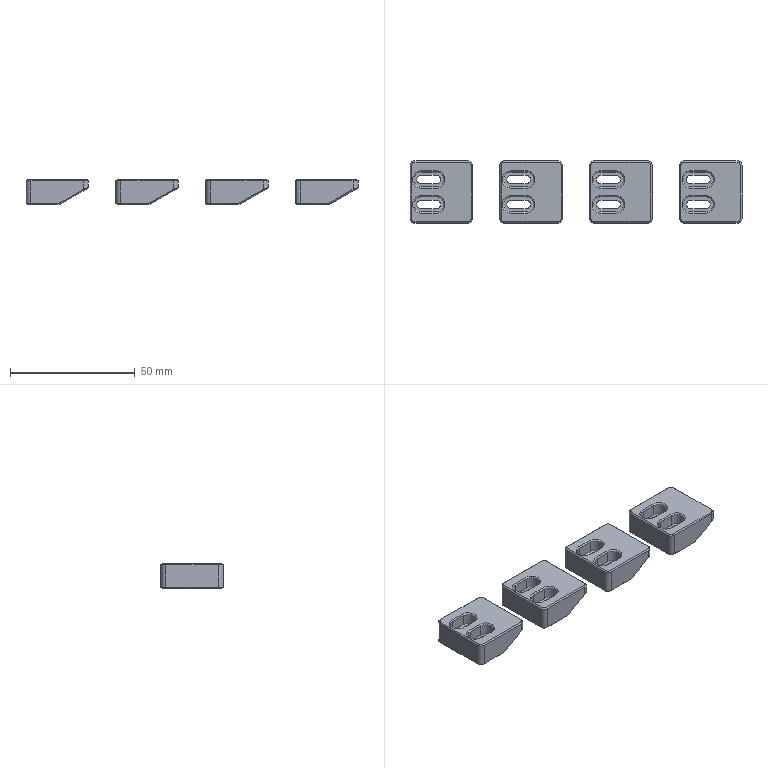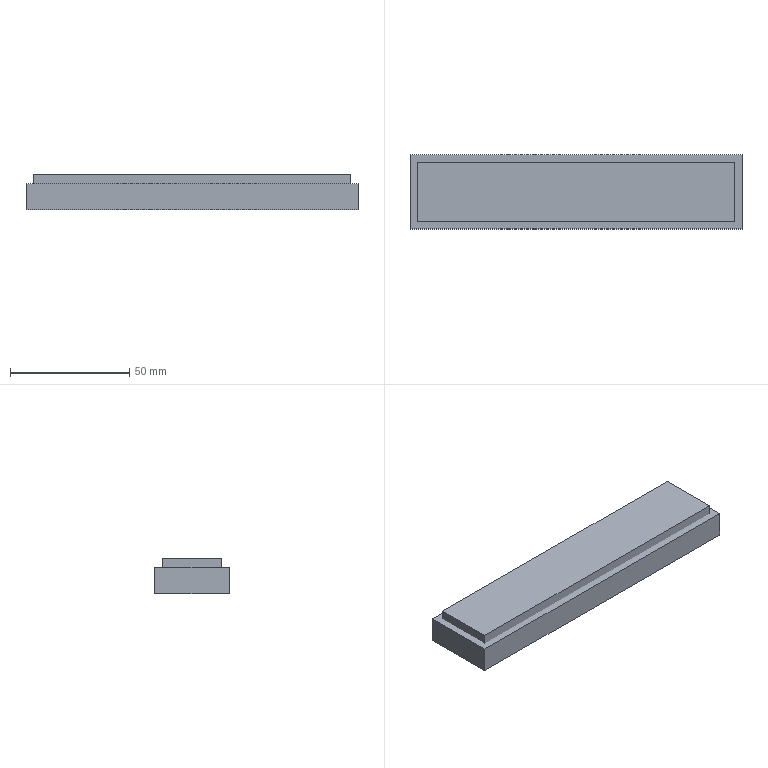CAM job | NX | 3-axis milling | part box 133 x 25 x 10 mm | stock box 139 x 31 x 15 mm
Tools:
number,name,description,diameter,corner_radius,flute_length,length,flutes
19,D80,Milling Tool-5 Parameters,80.0,0.0,50.0,75.0,2
15,D10,Milling Tool-5 Parameters,10.0,0.0,50.0,75.0,2
14,D10JING,Milling Tool-5 Parameters,10.0,0.0,50.0,75.0,2
16,D3,Milling Tool-5 Parameters,3.0,0.0,50.0,75.0,2
17,D4R0.5,Milling Tool-5 Parameters,4.0,0.5,50.0,75.0,2
1,D6A45,Milling Tool-5 Parameters,6.0,0.0,50.0,75.0,2
11,D4,Milling Tool-5 Parameters,4.0,0.0,50.0,75.0,2
Operations:
program,operation,operation_type,tool,method,geometry_group,spindle_rpm,surface_speed,feed_per_tooth,feed_cut,feed_plunge,cut_length_mm,path_length_mm,cut_time_min,machine_time_min
1,FLOOR_WALL,VolumeBased25DMillingOperation,D80,METHOD,A,6500.0,1633.0,0.1154,1500.0,100.0,231.0,285.0,0.154,0.1594
1,ZLEVEL_PROFILE,ZLevelMilling,D10,METHOD,A,9500.0,298.0,0.1316,2500.0,100.0,8567.78,8991.096,3.427,3.469
1,ZLEVEL_PROFILE_COPY_1_COPY_COPY_1,ZLevelMilling,D10JING,METHOD,A,9500.0,298.0,0.0632,1200.0,1000.0,541.463,994.087,0.4536,0.4989
1,ZLEVEL_PROFILE_COPY,ZLevelMilling,D3,METHOD,A,9500.0,89.0,0.0711,1350.0,100.0,2428.768,3072.315,1.799,1.863
1,ZLEVEL_PROFILE_1,ZLevelMilling,D4R0.5,METHOD,A,9500.0,119.0,0.1842,3500.0,1000.0,19412.518,19846.833,5.554,5.598
1,PLANAR_MILL_COPY_COPY_COPY_COPY_COPY_COPY_1,PlanarMilling,D6A45,METHOD,A,9500.0,179.0,0.0658,1250.0,100.0,421.184,770.38,0.3369,0.3719
1,PLANAR_MILL_COPY_COPY_COPY_COPY_COPY_COPY_1_COPY,PlanarMilling,D6A45,METHOD,A,9500.0,179.0,0.0658,1250.0,100.0,205.468,822.591,0.1644,0.2261
2,FLOOR_WALL_COPY,VolumeBased25DMillingOperation,D80,METHOD,B,6500.0,1633.0,0.1154,1500.0,100.0,1125.0,2251.001,0.75,0.8626
2,ZLEVEL_PROFILE_COPY_COPY,ZLevelMilling,D4,METHOD,B,9500.0,89.0,0.0711,1350.0,100.0,2873.971,3531.2,2.129,2.195
2,PLANAR_MILL_COPY_COPY_COPY_COPY_COPY_COPY_1_COPY_1,PlanarMilling,D6A45,METHOD,B,9500.0,179.0,0.0658,1250.0,100.0,681.628,1576.361,0.5453,0.6348